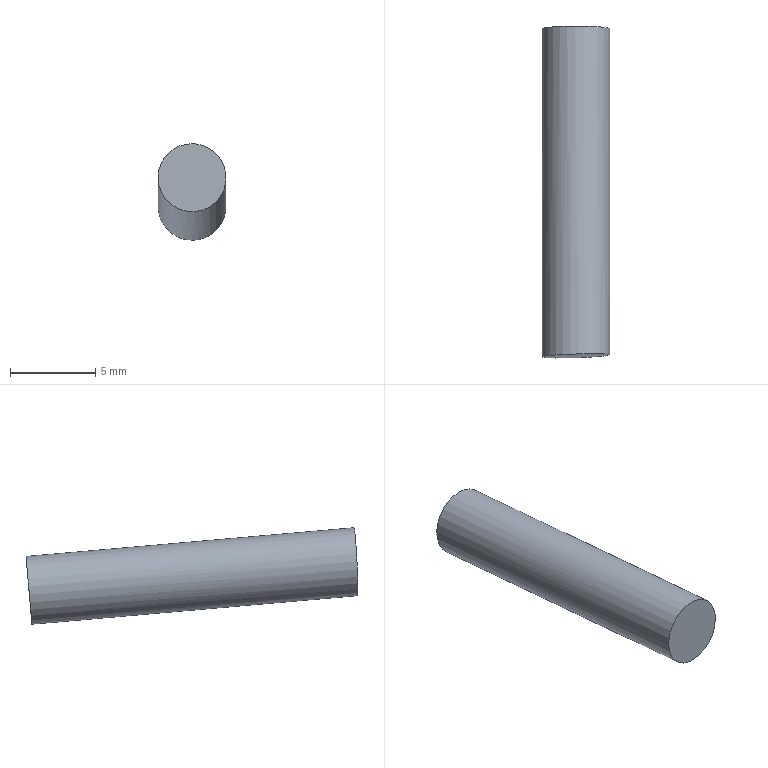Part | NX | features solid 2 | 1 solid | 3 faces | box 4 x 19.493 x 5.67 mm | volume 242.117 mm3 | plane 2 | cylinder 1 | commonest cylinder face diameters 4 x1
STEP:
#1=CARTESIAN_POINT('',(-242.835,-39.501,-43.97));
#2=VERTEX_POINT('',#1);
#3=CARTESIAN_POINT('',(-242.835,-39.326,-41.978));
#4=DIRECTION('',(0.,-0.9962,0.08716));
#5=DIRECTION('',(0.,-0.08716,-0.9962));
#6=AXIS2_PLACEMENT_3D('',#3,#4,#5);
#7=CIRCLE('',#6,2.);
#8=EDGE_CURVE('',#2,#2,#7,.T.);
#9=ORIENTED_EDGE('',*,*,#8,.F.);
#10=EDGE_LOOP('',(#9));
#11=FACE_BOUND('',#10,.T.);
#12=CARTESIAN_POINT('',(-228.366,-38.62,-33.907));
#13=DIRECTION('',(0.,-0.9962,0.08716));
#14=DIRECTION('',(0.,-0.08716,-0.9962));
#15=AXIS2_PLACEMENT_3D('',#12,#13,#14);
#16=PLANE('',#15);
#17=ADVANCED_FACE('',(#11),#16,.F.);
#18=CARTESIAN_POINT('',(-241.455,-58.552,-41.749));
#19=VERTEX_POINT('',#18);
#20=CARTESIAN_POINT('',(-242.835,-58.52,-40.299));
#21=DIRECTION('',(-0.03252,0.9981,-0.05307));
#22=DIRECTION('',(0.6892,-0.01607,-0.7244));
#23=AXIS2_PLACEMENT_3D('',#20,#21,#22);
#24=ELLIPSE('',#23,2.002,2.);
#25=EDGE_CURVE('',#19,#19,#24,.T.);
#26=ORIENTED_EDGE('',*,*,#25,.F.);
#27=EDGE_LOOP('',(#26));
#28=FACE_BOUND('',#27,.T.);
#29=CARTESIAN_POINT('',(-422.194,-57.948,80.353));
#30=DIRECTION('',(-0.03252,0.9981,-0.05307));
#31=DIRECTION('',(0.05223,-0.05133,-0.9973));
#32=AXIS2_PLACEMENT_3D('',#29,#30,#31);
#33=PLANE('',#32);
#34=ADVANCED_FACE('',(#28),#33,.F.);
#35=ORIENTED_EDGE('',*,*,#8,.T.);
#36=EDGE_LOOP('',(#35));
#37=FACE_BOUND('',#36,.T.);
#38=ORIENTED_EDGE('',*,*,#25,.T.);
#39=EDGE_LOOP('',(#38));
#40=FACE_BOUND('',#39,.T.);
#41=CARTESIAN_POINT('',(-242.835,-59.174,-40.241));
#42=DIRECTION('',(0.,0.9962,-0.08716));
#43=DIRECTION('',(1.,0.,0.));
#44=AXIS2_PLACEMENT_3D('',#41,#42,#43);
#45=CYLINDRICAL_SURFACE('',#44,2.);
#46=ADVANCED_FACE('',(#37,#40),#45,.T.);
#47=CLOSED_SHELL('',(#17,#34,#46));
#48=MANIFOLD_SOLID_BREP('',#47);
#49=(LENGTH_UNIT()NAMED_UNIT(*)SI_UNIT(.MILLI.,.METRE.));
#50=UNCERTAINTY_MEASURE_WITH_UNIT(LENGTH_MEASURE(0.00001),#49,'','');
#51=(NAMED_UNIT(*)PLANE_ANGLE_UNIT()SI_UNIT($,.RADIAN.));
#52=(NAMED_UNIT(*)SI_UNIT($,.STERADIAN.)SOLID_ANGLE_UNIT());
#53=(GEOMETRIC_REPRESENTATION_CONTEXT(3)GLOBAL_UNCERTAINTY_ASSIGNED_CONTEXT((#50))GLOBAL_UNIT_ASSIGNED_CONTEXT((#49,#51,#52))REPRESENTATION_CONTEXT('',''));
#54=ADVANCED_BREP_SHAPE_REPRESENTATION('',(#48),#53);